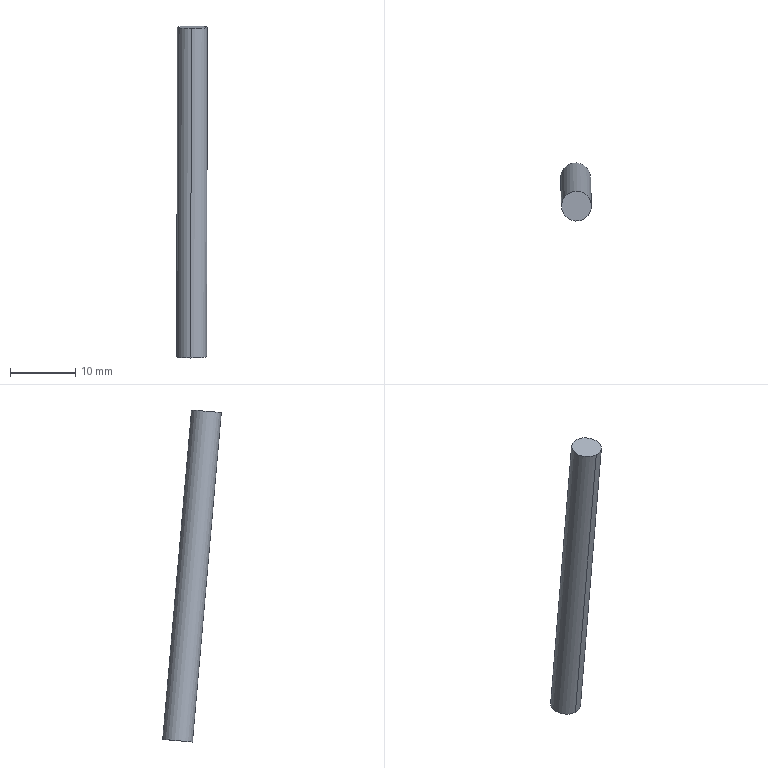Part | STEP file | 1_id870_x_t | 1 solid | 4 faces | box 4.715 x 9.009 x 51.008 mm | volume 844.246 mm3 | cylinder 2 | plane 2 | commonest cylinder face diameters 4.6 x2
STEP:
#1=CARTESIAN_POINT('',(0.,0.,0.));
#2=DIRECTION('',(0.,0.,1.));
#3=DIRECTION('',(1.,0.,0.));
#4=AXIS2_PLACEMENT_3D('',#1,#2,#3);
#5=CARTESIAN_POINT('',(972.469,347.424,-111.013));
#6=VERTEX_POINT('',#5);
#7=CARTESIAN_POINT('',(972.584,342.998,-60.406));
#8=VERTEX_POINT('',#7);
#9=CARTESIAN_POINT('',(972.469,347.424,-111.013));
#10=DIRECTION('',(0.002266,-0.08713,0.9962));
#11=VECTOR('',#10,1.);
#12=LINE('',#9,#11);
#13=CARTESIAN_POINT('',(972.623,349.71,-110.813));
#14=DIRECTION('',(0.002266,-0.08713,0.9962));
#15=DIRECTION('',(0.06685,0.994,0.08678));
#16=AXIS2_PLACEMENT_3D('',#13,#14,#15);
#17=CYLINDRICAL_SURFACE('',#16,2.3);
#18=CARTESIAN_POINT('',(3.142,0.));
#19=DIRECTION('',(0.,1.));
#20=VECTOR('',#19,1.);
#21=LINE('',#18,#20);
#22=(GEOMETRIC_REPRESENTATION_CONTEXT(2)PARAMETRIC_REPRESENTATION_CONTEXT()REPRESENTATION_CONTEXT('',''));
#23=DEFINITIONAL_REPRESENTATION('',(#21),#22);
#24=PCURVE('',#17,#23);
#25=CARTESIAN_POINT('',(972.623,349.71,-110.813));
#26=DIRECTION('',(0.002266,-0.08713,0.9962));
#27=DIRECTION('',(0.06685,0.994,0.08678));
#28=AXIS2_PLACEMENT_3D('',#25,#26,#27);
#29=CYLINDRICAL_SURFACE('',#28,2.3);
#30=CARTESIAN_POINT('',(3.142,0.));
#31=DIRECTION('',(0.,1.));
#32=VECTOR('',#31,1.);
#33=LINE('',#30,#32);
#34=(GEOMETRIC_REPRESENTATION_CONTEXT(2)PARAMETRIC_REPRESENTATION_CONTEXT()REPRESENTATION_CONTEXT('',''));
#35=DEFINITIONAL_REPRESENTATION('',(#33),#34);
#36=PCURVE('',#29,#35);
#37=SURFACE_CURVE('',#12,(#24,#36),.PCURVE_S1.);
#38=EDGE_CURVE('',#6,#8,#37,.T.);
#39=ORIENTED_EDGE('',*,*,#38,.F.);
#40=CARTESIAN_POINT('',(972.777,351.996,-110.614));
#41=VERTEX_POINT('',#40);
#42=CARTESIAN_POINT('',(972.623,349.71,-110.813));
#43=DIRECTION('',(-0.002266,0.08713,-0.9962));
#44=DIRECTION('',(0.06685,0.994,0.08678));
#45=AXIS2_PLACEMENT_3D('',#42,#43,#44);
#46=CIRCLE('',#45,2.3);
#47=CARTESIAN_POINT('',(6.283,0.));
#48=DIRECTION('',(-1.,0.));
#49=VECTOR('',#48,1.);
#50=LINE('',#47,#49);
#51=(GEOMETRIC_REPRESENTATION_CONTEXT(2)PARAMETRIC_REPRESENTATION_CONTEXT()REPRESENTATION_CONTEXT('',''));
#52=DEFINITIONAL_REPRESENTATION('',(#50),#51);
#53=PCURVE('',#17,#52);
#54=CARTESIAN_POINT('',(972.623,349.71,-110.813));
#55=DIRECTION('',(-0.002266,0.08713,-0.9962));
#56=DIRECTION('',(0.8426,0.5366,0.04501));
#57=AXIS2_PLACEMENT_3D('',#54,#55,#56);
#58=PLANE('',#57);
#59=CARTESIAN_POINT('',(0.,0.));
#60=DIRECTION('',(0.5936,-0.8047));
#61=AXIS2_PLACEMENT_2D('',#59,#60);
#62=CIRCLE('',#61,2.3);
#63=(GEOMETRIC_REPRESENTATION_CONTEXT(2)PARAMETRIC_REPRESENTATION_CONTEXT()REPRESENTATION_CONTEXT('',''));
#64=DEFINITIONAL_REPRESENTATION('',(#62),#63);
#65=PCURVE('',#58,#64);
#66=SURFACE_CURVE('',#46,(#53,#65),.PCURVE_S1.);
#67=EDGE_CURVE('',#41,#6,#66,.T.);
#68=ORIENTED_EDGE('',*,*,#67,.F.);
#69=CARTESIAN_POINT('',(972.892,347.57,-60.007));
#70=VERTEX_POINT('',#69);
#71=CARTESIAN_POINT('',(972.777,351.996,-110.614));
#72=DIRECTION('',(-0.002266,0.08713,-0.9962));
#73=VECTOR('',#72,1.);
#74=LINE('',#71,#73);
#75=CARTESIAN_POINT('',(6.283,0.));
#76=DIRECTION('',(0.,-1.));
#77=VECTOR('',#76,1.);
#78=LINE('',#75,#77);
#79=(GEOMETRIC_REPRESENTATION_CONTEXT(2)PARAMETRIC_REPRESENTATION_CONTEXT()REPRESENTATION_CONTEXT('',''));
#80=DEFINITIONAL_REPRESENTATION('',(#78),#79);
#81=PCURVE('',#17,#80);
#82=CARTESIAN_POINT('',(0.,0.));
#83=DIRECTION('',(0.,-1.));
#84=VECTOR('',#83,1.);
#85=LINE('',#82,#84);
#86=(GEOMETRIC_REPRESENTATION_CONTEXT(2)PARAMETRIC_REPRESENTATION_CONTEXT()REPRESENTATION_CONTEXT('',''));
#87=DEFINITIONAL_REPRESENTATION('',(#85),#86);
#88=PCURVE('',#29,#87);
#89=SURFACE_CURVE('',#74,(#81,#88),.PCURVE_S1.);
#90=EDGE_CURVE('',#70,#41,#89,.T.);
#91=ORIENTED_EDGE('',*,*,#90,.F.);
#92=CARTESIAN_POINT('',(972.738,345.284,-60.206));
#93=DIRECTION('',(0.002266,-0.08713,0.9962));
#94=DIRECTION('',(-0.06685,-0.994,-0.08678));
#95=AXIS2_PLACEMENT_3D('',#92,#93,#94);
#96=CIRCLE('',#95,2.3);
#97=CARTESIAN_POINT('',(3.142,50.8));
#98=DIRECTION('',(1.,0.));
#99=VECTOR('',#98,1.);
#100=LINE('',#97,#99);
#101=(GEOMETRIC_REPRESENTATION_CONTEXT(2)PARAMETRIC_REPRESENTATION_CONTEXT()REPRESENTATION_CONTEXT('',''));
#102=DEFINITIONAL_REPRESENTATION('',(#100),#101);
#103=PCURVE('',#17,#102);
#104=CARTESIAN_POINT('',(972.738,345.284,-60.206));
#105=DIRECTION('',(-0.002266,0.08713,-0.9962));
#106=DIRECTION('',(0.8426,0.5366,0.04501));
#107=AXIS2_PLACEMENT_3D('',#104,#105,#106);
#108=PLANE('',#107);
#109=CARTESIAN_POINT('',(-1.365,1.851));
#110=CARTESIAN_POINT('',(1.841,4.216));
#111=CARTESIAN_POINT('',(2.286,0.2569));
#112=CARTESIAN_POINT('',(2.731,-3.702));
#113=CARTESIAN_POINT('',(-0.9203,-2.108));
#114=CARTESIAN_POINT('',(-4.571,-0.5139));
#115=CARTESIAN_POINT('',(-1.365,1.851));
#116=(BOUNDED_CURVE()B_SPLINE_CURVE(2,(#109,#110,#111,#112,#113,#114,#115),.UNSPECIFIED.,.T.,.F.)B_SPLINE_CURVE_WITH_KNOTS((1,2,2,2,2,1),(-2.094,0.,2.094,4.189,6.283,8.378),.UNSPECIFIED.)CURVE()GEOMETRIC_REPRESENTATION_ITEM()RATIONAL_B_SPLINE_CURVE((1.,0.5,1.,0.5,1.,0.5,1.))REPRESENTATION_ITEM(''));
#117=(GEOMETRIC_REPRESENTATION_CONTEXT(2)PARAMETRIC_REPRESENTATION_CONTEXT()REPRESENTATION_CONTEXT('',''));
#118=DEFINITIONAL_REPRESENTATION('',(#116),#117);
#119=PCURVE('',#108,#118);
#120=SURFACE_CURVE('',#96,(#103,#119),.PCURVE_S1.);
#121=EDGE_CURVE('',#8,#70,#120,.T.);
#122=ORIENTED_EDGE('',*,*,#121,.F.);
#123=EDGE_LOOP('',(#39,#68,#91,#122));
#124=FACE_BOUND('',#123,.T.);
#125=ADVANCED_FACE('',(#124),#17,.T.);
#126=ORIENTED_EDGE('',*,*,#121,.T.);
#127=CARTESIAN_POINT('',(972.738,345.284,-60.206));
#128=DIRECTION('',(0.002266,-0.08713,0.9962));
#129=DIRECTION('',(0.06685,0.994,0.08678));
#130=AXIS2_PLACEMENT_3D('',#127,#128,#129);
#131=CIRCLE('',#130,2.3);
#132=CARTESIAN_POINT('',(1.365,-1.851));
#133=CARTESIAN_POINT('',(-1.841,-4.216));
#134=CARTESIAN_POINT('',(-2.286,-0.2569));
#135=CARTESIAN_POINT('',(-2.731,3.702));
#136=CARTESIAN_POINT('',(0.9203,2.108));
#137=CARTESIAN_POINT('',(4.571,0.5139));
#138=CARTESIAN_POINT('',(1.365,-1.851));
#139=(BOUNDED_CURVE()B_SPLINE_CURVE(2,(#132,#133,#134,#135,#136,#137,#138),.UNSPECIFIED.,.T.,.F.)B_SPLINE_CURVE_WITH_KNOTS((1,2,2,2,2,1),(-2.094,0.,2.094,4.189,6.283,8.378),.UNSPECIFIED.)CURVE()GEOMETRIC_REPRESENTATION_ITEM()RATIONAL_B_SPLINE_CURVE((1.,0.5,1.,0.5,1.,0.5,1.))REPRESENTATION_ITEM(''));
#140=(GEOMETRIC_REPRESENTATION_CONTEXT(2)PARAMETRIC_REPRESENTATION_CONTEXT()REPRESENTATION_CONTEXT('',''));
#141=DEFINITIONAL_REPRESENTATION('',(#139),#140);
#142=PCURVE('',#108,#141);
#143=CARTESIAN_POINT('',(0.,50.8));
#144=DIRECTION('',(1.,0.));
#145=VECTOR('',#144,1.);
#146=LINE('',#143,#145);
#147=(GEOMETRIC_REPRESENTATION_CONTEXT(2)PARAMETRIC_REPRESENTATION_CONTEXT()REPRESENTATION_CONTEXT('',''));
#148=DEFINITIONAL_REPRESENTATION('',(#146),#147);
#149=PCURVE('',#29,#148);
#150=SURFACE_CURVE('',#131,(#142,#149),.PCURVE_S1.);
#151=EDGE_CURVE('',#70,#8,#150,.T.);
#152=ORIENTED_EDGE('',*,*,#151,.T.);
#153=EDGE_LOOP('',(#126,#152));
#154=FACE_BOUND('',#153,.T.);
#155=ADVANCED_FACE('',(#154),#108,.F.);
#156=ORIENTED_EDGE('',*,*,#90,.T.);
#157=CARTESIAN_POINT('',(972.623,349.71,-110.813));
#158=DIRECTION('',(-0.002266,0.08713,-0.9962));
#159=DIRECTION('',(-0.06685,-0.994,-0.08678));
#160=AXIS2_PLACEMENT_3D('',#157,#158,#159);
#161=CIRCLE('',#160,2.3);
#162=CARTESIAN_POINT('',(3.142,0.));
#163=DIRECTION('',(-1.,0.));
#164=VECTOR('',#163,1.);
#165=LINE('',#162,#164);
#166=(GEOMETRIC_REPRESENTATION_CONTEXT(2)PARAMETRIC_REPRESENTATION_CONTEXT()REPRESENTATION_CONTEXT('',''));
#167=DEFINITIONAL_REPRESENTATION('',(#165),#166);
#168=PCURVE('',#29,#167);
#169=CARTESIAN_POINT('',(0.,0.));
#170=DIRECTION('',(-0.5936,0.8047));
#171=AXIS2_PLACEMENT_2D('',#169,#170);
#172=CIRCLE('',#171,2.3);
#173=(GEOMETRIC_REPRESENTATION_CONTEXT(2)PARAMETRIC_REPRESENTATION_CONTEXT()REPRESENTATION_CONTEXT('',''));
#174=DEFINITIONAL_REPRESENTATION('',(#172),#173);
#175=PCURVE('',#58,#174);
#176=SURFACE_CURVE('',#161,(#168,#175),.PCURVE_S1.);
#177=EDGE_CURVE('',#6,#41,#176,.T.);
#178=ORIENTED_EDGE('',*,*,#177,.F.);
#179=ORIENTED_EDGE('',*,*,#38,.T.);
#180=ORIENTED_EDGE('',*,*,#151,.F.);
#181=EDGE_LOOP('',(#156,#178,#179,#180));
#182=FACE_BOUND('',#181,.T.);
#183=ADVANCED_FACE('',(#182),#29,.T.);
#184=ORIENTED_EDGE('',*,*,#177,.T.);
#185=ORIENTED_EDGE('',*,*,#67,.T.);
#186=EDGE_LOOP('',(#184,#185));
#187=FACE_BOUND('',#186,.T.);
#188=ADVANCED_FACE('',(#187),#58,.T.);
#189=CLOSED_SHELL('',(#125,#155,#183,#188));
#190=MANIFOLD_SOLID_BREP('',#189);
#191=(LENGTH_UNIT()NAMED_UNIT(*)SI_UNIT(.MILLI.,.METRE.));
#192=UNCERTAINTY_MEASURE_WITH_UNIT(LENGTH_MEASURE(0.0000001),#191,'','');
#193=(NAMED_UNIT(*)PLANE_ANGLE_UNIT()SI_UNIT($,.RADIAN.));
#194=(NAMED_UNIT(*)SI_UNIT($,.STERADIAN.)SOLID_ANGLE_UNIT());
#195=(GEOMETRIC_REPRESENTATION_CONTEXT(3)GLOBAL_UNCERTAINTY_ASSIGNED_CONTEXT((#192))GLOBAL_UNIT_ASSIGNED_CONTEXT((#191,#193,#194))REPRESENTATION_CONTEXT('',''));
#196=ADVANCED_BREP_SHAPE_REPRESENTATION('',(#4,#190),#195);